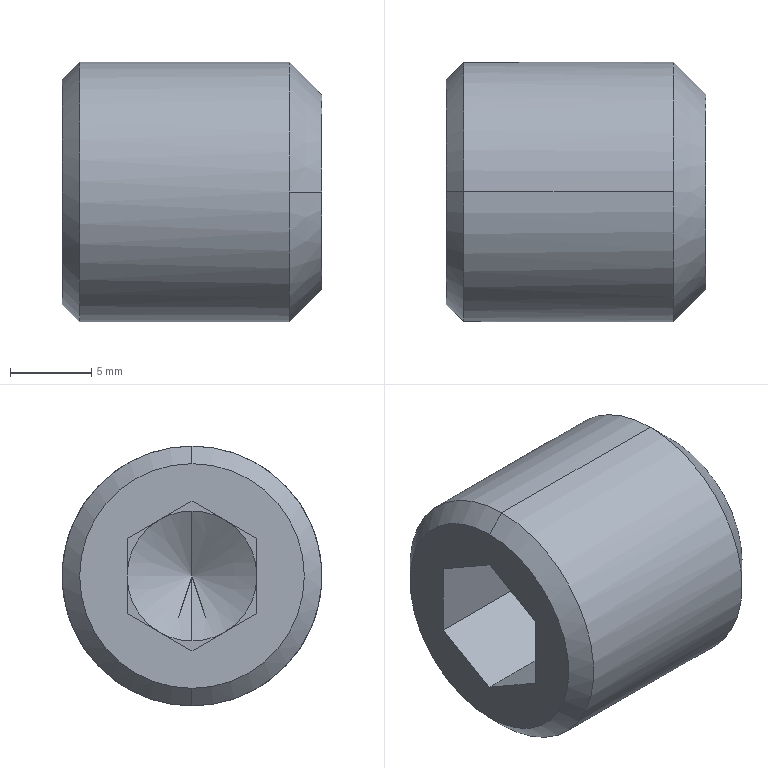Part | SolidWorks | features BaseBody 1 | 1 solid | 22 faces | box 16 x 16 x 16 mm | volume 2703 mm3 | plane 14 | cone 6 | cylinder 2 | commonest cylinder face diameters 16 x2
STEP:
#1=CARTESIAN_POINT('',(14.,8.,0.));
#2=VERTEX_POINT('',#1);
#3=CARTESIAN_POINT('',(14.,0.,-8.));
#4=VERTEX_POINT('',#3);
#5=CARTESIAN_POINT('',(14.,0.,0.));
#6=DIRECTION('',(-1.,0.,0.));
#7=DIRECTION('',(0.,0.,1.));
#8=AXIS2_PLACEMENT_3D('',#5,#6,#7);
#9=CIRCLE('',#8,8.);
#10=EDGE_CURVE('',#2,#4,#9,.T.);
#11=ORIENTED_EDGE('',*,*,#10,.T.);
#12=CARTESIAN_POINT('',(1.083,0.,-8.));
#13=VERTEX_POINT('',#12);
#14=CARTESIAN_POINT('',(-10.745,0.,-8.));
#15=DIRECTION('',(-1.,0.,0.));
#16=VECTOR('',#15,1000.);
#17=LINE('',#14,#16);
#18=EDGE_CURVE('',#4,#13,#17,.T.);
#19=ORIENTED_EDGE('',*,*,#18,.T.);
#20=CARTESIAN_POINT('',(1.083,0.,8.));
#21=VERTEX_POINT('',#20);
#22=CARTESIAN_POINT('',(1.083,0.,0.));
#23=DIRECTION('',(1.,0.,0.));
#24=DIRECTION('',(0.,0.,1.));
#25=AXIS2_PLACEMENT_3D('',#22,#23,#24);
#26=CIRCLE('',#25,8.);
#27=EDGE_CURVE('',#13,#21,#26,.T.);
#28=ORIENTED_EDGE('',*,*,#27,.T.);
#29=CARTESIAN_POINT('',(14.,0.,8.));
#30=VERTEX_POINT('',#29);
#31=CARTESIAN_POINT('',(-10.745,0.,8.));
#32=DIRECTION('',(-1.,0.,0.));
#33=VECTOR('',#32,1000.);
#34=LINE('',#31,#33);
#35=EDGE_CURVE('',#30,#21,#34,.T.);
#36=ORIENTED_EDGE('',*,*,#35,.F.);
#37=CARTESIAN_POINT('',(14.,0.,0.));
#38=DIRECTION('',(-1.,0.,0.));
#39=DIRECTION('',(0.,0.,1.));
#40=AXIS2_PLACEMENT_3D('',#37,#38,#39);
#41=CIRCLE('',#40,8.);
#42=EDGE_CURVE('',#30,#2,#41,.T.);
#43=ORIENTED_EDGE('',*,*,#42,.T.);
#44=EDGE_LOOP('',(#11,#19,#28,#36,#43));
#45=FACE_OUTER_BOUND('',#44,.T.);
#46=CARTESIAN_POINT('',(-10.745,0.,0.));
#47=DIRECTION('',(-1.,0.,0.));
#48=DIRECTION('',(0.,0.,1.));
#49=AXIS2_PLACEMENT_3D('',#46,#47,#48);
#50=CYLINDRICAL_SURFACE('',#49,8.);
#51=ADVANCED_FACE('',(#45),#50,.T.);
#52=CARTESIAN_POINT('',(16.,-6.,0.));
#53=VERTEX_POINT('',#52);
#54=CARTESIAN_POINT('',(16.,6.,0.));
#55=VERTEX_POINT('',#54);
#56=CARTESIAN_POINT('',(16.,0.,0.));
#57=DIRECTION('',(-1.,0.,0.));
#58=DIRECTION('',(0.,-1.,0.));
#59=AXIS2_PLACEMENT_3D('',#56,#57,#58);
#60=CIRCLE('',#59,6.);
#61=EDGE_CURVE('',#53,#55,#60,.T.);
#62=ORIENTED_EDGE('',*,*,#61,.T.);
#63=CARTESIAN_POINT('',(14.,8.,0.));
#64=DIRECTION('',(-0.7071,0.7071,0.));
#65=VECTOR('',#64,1000.);
#66=LINE('',#63,#65);
#67=EDGE_CURVE('',#55,#2,#66,.T.);
#68=ORIENTED_EDGE('',*,*,#67,.T.);
#69=ORIENTED_EDGE('',*,*,#42,.F.);
#70=CARTESIAN_POINT('',(14.,-8.,0.));
#71=VERTEX_POINT('',#70);
#72=CARTESIAN_POINT('',(14.,0.,0.));
#73=DIRECTION('',(-1.,0.,0.));
#74=DIRECTION('',(0.,0.,1.));
#75=AXIS2_PLACEMENT_3D('',#72,#73,#74);
#76=CIRCLE('',#75,8.);
#77=EDGE_CURVE('',#71,#30,#76,.T.);
#78=ORIENTED_EDGE('',*,*,#77,.F.);
#79=CARTESIAN_POINT('',(14.,-8.,0.));
#80=DIRECTION('',(-0.7071,-0.7071,0.));
#81=VECTOR('',#80,1000.);
#82=LINE('',#79,#81);
#83=EDGE_CURVE('',#53,#71,#82,.T.);
#84=ORIENTED_EDGE('',*,*,#83,.F.);
#85=EDGE_LOOP('',(#62,#68,#69,#78,#84));
#86=FACE_OUTER_BOUND('',#85,.T.);
#87=CARTESIAN_POINT('',(14.,0.,0.));
#88=DIRECTION('',(-1.,0.,0.));
#89=DIRECTION('',(0.,-1.,0.));
#90=AXIS2_PLACEMENT_3D('',#87,#88,#89);
#91=CONICAL_SURFACE('',#90,8.,0.7854);
#92=ADVANCED_FACE('',(#86),#91,.T.);
#93=CARTESIAN_POINT('',(0.,0.,-6.918));
#94=VERTEX_POINT('',#93);
#95=CARTESIAN_POINT('',(0.,0.,6.918));
#96=VERTEX_POINT('',#95);
#97=CARTESIAN_POINT('',(0.,0.,0.));
#98=DIRECTION('',(1.,0.,0.));
#99=DIRECTION('',(0.,0.,-1.));
#100=AXIS2_PLACEMENT_3D('',#97,#98,#99);
#101=CIRCLE('',#100,6.918);
#102=EDGE_CURVE('',#94,#96,#101,.T.);
#103=ORIENTED_EDGE('',*,*,#102,.T.);
#104=CARTESIAN_POINT('',(1.083,0.,8.));
#105=DIRECTION('',(0.7071,0.,0.7071));
#106=VECTOR('',#105,1000.);
#107=LINE('',#104,#106);
#108=EDGE_CURVE('',#96,#21,#107,.T.);
#109=ORIENTED_EDGE('',*,*,#108,.T.);
#110=ORIENTED_EDGE('',*,*,#27,.F.);
#111=CARTESIAN_POINT('',(1.083,0.,-8.));
#112=DIRECTION('',(0.7071,0.,-0.7071));
#113=VECTOR('',#112,1000.);
#114=LINE('',#111,#113);
#115=EDGE_CURVE('',#94,#13,#114,.T.);
#116=ORIENTED_EDGE('',*,*,#115,.F.);
#117=EDGE_LOOP('',(#103,#109,#110,#116));
#118=FACE_OUTER_BOUND('',#117,.T.);
#119=CARTESIAN_POINT('',(1.083,0.,0.));
#120=DIRECTION('',(1.,0.,0.));
#121=DIRECTION('',(0.,0.,-1.));
#122=AXIS2_PLACEMENT_3D('',#119,#120,#121);
#123=CONICAL_SURFACE('',#122,8.,0.7854);
#124=ADVANCED_FACE('',(#118),#123,.T.);
#125=CARTESIAN_POINT('',(8.709,0.,0.));
#126=VERTEX_POINT('',#125);
#127=CARTESIAN_POINT('',(6.4,0.,4.));
#128=VERTEX_POINT('',#127);
#129=CARTESIAN_POINT('',(6.4,0.,4.));
#130=DIRECTION('',(-0.5,0.,0.866));
#131=VECTOR('',#130,1000.);
#132=LINE('',#129,#131);
#133=EDGE_CURVE('',#126,#128,#132,.T.);
#134=ORIENTED_EDGE('',*,*,#133,.F.);
#135=CARTESIAN_POINT('',(6.4,0.,-4.));
#136=VERTEX_POINT('',#135);
#137=CARTESIAN_POINT('',(6.4,0.,-4.));
#138=DIRECTION('',(-0.5,0.,-0.866));
#139=VECTOR('',#138,1000.);
#140=LINE('',#137,#139);
#141=EDGE_CURVE('',#126,#136,#140,.T.);
#142=ORIENTED_EDGE('',*,*,#141,.T.);
#143=CARTESIAN_POINT('',(6.4,-2.,-3.464));
#144=VERTEX_POINT('',#143);
#145=CARTESIAN_POINT('',(6.4,0.,0.));
#146=DIRECTION('',(1.,0.,0.));
#147=DIRECTION('',(0.,0.,1.));
#148=AXIS2_PLACEMENT_3D('',#145,#146,#147);
#149=CIRCLE('',#148,4.);
#150=EDGE_CURVE('',#144,#136,#149,.T.);
#151=ORIENTED_EDGE('',*,*,#150,.F.);
#152=CARTESIAN_POINT('',(6.4,-4.,0.));
#153=VERTEX_POINT('',#152);
#154=CARTESIAN_POINT('',(6.4,0.,0.));
#155=DIRECTION('',(1.,0.,0.));
#156=DIRECTION('',(0.,0.,1.));
#157=AXIS2_PLACEMENT_3D('',#154,#155,#156);
#158=CIRCLE('',#157,4.);
#159=EDGE_CURVE('',#153,#144,#158,.T.);
#160=ORIENTED_EDGE('',*,*,#159,.F.);
#161=CARTESIAN_POINT('',(6.4,-2.,3.464));
#162=VERTEX_POINT('',#161);
#163=CARTESIAN_POINT('',(6.4,0.,0.));
#164=DIRECTION('',(1.,0.,0.));
#165=DIRECTION('',(0.,0.,1.));
#166=AXIS2_PLACEMENT_3D('',#163,#164,#165);
#167=CIRCLE('',#166,4.);
#168=EDGE_CURVE('',#162,#153,#167,.T.);
#169=ORIENTED_EDGE('',*,*,#168,.F.);
#170=CARTESIAN_POINT('',(6.4,0.,0.));
#171=DIRECTION('',(1.,0.,0.));
#172=DIRECTION('',(0.,0.,1.));
#173=AXIS2_PLACEMENT_3D('',#170,#171,#172);
#174=CIRCLE('',#173,4.);
#175=EDGE_CURVE('',#128,#162,#174,.T.);
#176=ORIENTED_EDGE('',*,*,#175,.F.);
#177=EDGE_LOOP('',(#134,#142,#151,#160,#169,#176));
#178=FACE_OUTER_BOUND('',#177,.T.);
#179=CARTESIAN_POINT('',(6.4,0.,0.));
#180=DIRECTION('',(-1.,0.,0.));
#181=DIRECTION('',(0.,0.,1.));
#182=AXIS2_PLACEMENT_3D('',#179,#180,#181);
#183=CONICAL_SURFACE('',#182,4.,1.047);
#184=ADVANCED_FACE('',(#178),#183,.F.);
#185=ORIENTED_EDGE('',*,*,#18,.F.);
#186=CARTESIAN_POINT('',(14.,0.,0.));
#187=DIRECTION('',(-1.,0.,0.));
#188=DIRECTION('',(0.,0.,1.));
#189=AXIS2_PLACEMENT_3D('',#186,#187,#188);
#190=CIRCLE('',#189,8.);
#191=EDGE_CURVE('',#4,#71,#190,.T.);
#192=ORIENTED_EDGE('',*,*,#191,.T.);
#193=ORIENTED_EDGE('',*,*,#77,.T.);
#194=ORIENTED_EDGE('',*,*,#35,.T.);
#195=CARTESIAN_POINT('',(1.083,0.,0.));
#196=DIRECTION('',(1.,0.,0.));
#197=DIRECTION('',(0.,0.,1.));
#198=AXIS2_PLACEMENT_3D('',#195,#196,#197);
#199=CIRCLE('',#198,8.);
#200=EDGE_CURVE('',#21,#13,#199,.T.);
#201=ORIENTED_EDGE('',*,*,#200,.T.);
#202=EDGE_LOOP('',(#185,#192,#193,#194,#201));
#203=FACE_OUTER_BOUND('',#202,.T.);
#204=CARTESIAN_POINT('',(-10.745,0.,0.));
#205=DIRECTION('',(-1.,0.,0.));
#206=DIRECTION('',(0.,0.,1.));
#207=AXIS2_PLACEMENT_3D('',#204,#205,#206);
#208=CYLINDRICAL_SURFACE('',#207,8.);
#209=ADVANCED_FACE('',(#203),#208,.T.);
#210=ORIENTED_EDGE('',*,*,#67,.F.);
#211=CARTESIAN_POINT('',(16.,0.,0.));
#212=DIRECTION('',(-1.,0.,0.));
#213=DIRECTION('',(0.,-1.,0.));
#214=AXIS2_PLACEMENT_3D('',#211,#212,#213);
#215=CIRCLE('',#214,6.);
#216=EDGE_CURVE('',#55,#53,#215,.T.);
#217=ORIENTED_EDGE('',*,*,#216,.T.);
#218=ORIENTED_EDGE('',*,*,#83,.T.);
#219=ORIENTED_EDGE('',*,*,#191,.F.);
#220=ORIENTED_EDGE('',*,*,#10,.F.);
#221=EDGE_LOOP('',(#210,#217,#218,#219,#220));
#222=FACE_OUTER_BOUND('',#221,.T.);
#223=CARTESIAN_POINT('',(14.,0.,0.));
#224=DIRECTION('',(-1.,0.,0.));
#225=DIRECTION('',(0.,-1.,0.));
#226=AXIS2_PLACEMENT_3D('',#223,#224,#225);
#227=CONICAL_SURFACE('',#226,8.,0.7854);
#228=ADVANCED_FACE('',(#222),#227,.T.);
#229=ORIENTED_EDGE('',*,*,#108,.F.);
#230=CARTESIAN_POINT('',(0.,0.,0.));
#231=DIRECTION('',(1.,0.,0.));
#232=DIRECTION('',(0.,0.,-1.));
#233=AXIS2_PLACEMENT_3D('',#230,#231,#232);
#234=CIRCLE('',#233,6.918);
#235=EDGE_CURVE('',#96,#94,#234,.T.);
#236=ORIENTED_EDGE('',*,*,#235,.T.);
#237=ORIENTED_EDGE('',*,*,#115,.T.);
#238=ORIENTED_EDGE('',*,*,#200,.F.);
#239=EDGE_LOOP('',(#229,#236,#237,#238));
#240=FACE_OUTER_BOUND('',#239,.T.);
#241=CARTESIAN_POINT('',(1.083,0.,0.));
#242=DIRECTION('',(1.,0.,0.));
#243=DIRECTION('',(0.,0.,-1.));
#244=AXIS2_PLACEMENT_3D('',#241,#242,#243);
#245=CONICAL_SURFACE('',#244,8.,0.7854);
#246=ADVANCED_FACE('',(#240),#245,.T.);
#247=ORIENTED_EDGE('',*,*,#61,.F.);
#248=ORIENTED_EDGE('',*,*,#216,.F.);
#249=EDGE_LOOP('',(#247,#248));
#250=FACE_OUTER_BOUND('',#249,.T.);
#251=CARTESIAN_POINT('',(16.,0.,0.));
#252=DIRECTION('',(-1.,0.,0.));
#253=DIRECTION('',(0.,0.,1.));
#254=AXIS2_PLACEMENT_3D('',#251,#252,#253);
#255=PLANE('',#254);
#256=ADVANCED_FACE('',(#250),#255,.F.);
#257=CARTESIAN_POINT('',(0.,-4.,-2.309));
#258=VERTEX_POINT('',#257);
#259=CARTESIAN_POINT('',(0.,-4.,2.309));
#260=VERTEX_POINT('',#259);
#261=CARTESIAN_POINT('',(0.,-4.,0.));
#262=DIRECTION('',(0.,0.,1.));
#263=VECTOR('',#262,1000.);
#264=LINE('',#261,#263);
#265=EDGE_CURVE('',#258,#260,#264,.T.);
#266=ORIENTED_EDGE('',*,*,#265,.F.);
#267=CARTESIAN_POINT('',(0.,0.,-4.619));
#268=VERTEX_POINT('',#267);
#269=CARTESIAN_POINT('',(0.,0.,-4.619));
#270=DIRECTION('',(0.,-0.866,0.5));
#271=VECTOR('',#270,1000.);
#272=LINE('',#269,#271);
#273=EDGE_CURVE('',#268,#258,#272,.T.);
#274=ORIENTED_EDGE('',*,*,#273,.F.);
#275=CARTESIAN_POINT('',(0.,4.,-2.309));
#276=VERTEX_POINT('',#275);
#277=CARTESIAN_POINT('',(0.,4.,-2.309));
#278=DIRECTION('',(0.,-0.866,-0.5));
#279=VECTOR('',#278,1000.);
#280=LINE('',#277,#279);
#281=EDGE_CURVE('',#276,#268,#280,.T.);
#282=ORIENTED_EDGE('',*,*,#281,.F.);
#283=CARTESIAN_POINT('',(0.,4.,2.309));
#284=VERTEX_POINT('',#283);
#285=CARTESIAN_POINT('',(0.,4.,0.));
#286=DIRECTION('',(0.,0.,-1.));
#287=VECTOR('',#286,1000.);
#288=LINE('',#285,#287);
#289=EDGE_CURVE('',#284,#276,#288,.T.);
#290=ORIENTED_EDGE('',*,*,#289,.F.);
#291=CARTESIAN_POINT('',(0.,0.,4.619));
#292=VERTEX_POINT('',#291);
#293=CARTESIAN_POINT('',(0.,0.,4.619));
#294=DIRECTION('',(0.,0.866,-0.5));
#295=VECTOR('',#294,1000.);
#296=LINE('',#293,#295);
#297=EDGE_CURVE('',#292,#284,#296,.T.);
#298=ORIENTED_EDGE('',*,*,#297,.F.);
#299=CARTESIAN_POINT('',(0.,-4.,2.309));
#300=DIRECTION('',(0.,0.866,0.5));
#301=VECTOR('',#300,1000.);
#302=LINE('',#299,#301);
#303=EDGE_CURVE('',#260,#292,#302,.T.);
#304=ORIENTED_EDGE('',*,*,#303,.F.);
#305=EDGE_LOOP('',(#266,#274,#282,#290,#298,#304));
#306=FACE_BOUND('',#305,.T.);
#307=ORIENTED_EDGE('',*,*,#102,.F.);
#308=ORIENTED_EDGE('',*,*,#235,.F.);
#309=EDGE_LOOP('',(#307,#308));
#310=FACE_OUTER_BOUND('',#309,.T.);
#311=CARTESIAN_POINT('',(0.,6.918,0.));
#312=DIRECTION('',(1.,0.,0.));
#313=DIRECTION('',(0.,0.,-1.));
#314=AXIS2_PLACEMENT_3D('',#311,#312,#313);
#315=PLANE('',#314);
#316=ADVANCED_FACE('',(#306,#310),#315,.F.);
#317=CARTESIAN_POINT('',(6.4,0.,4.619));
#318=VERTEX_POINT('',#317);
#319=CARTESIAN_POINT('',(6.4,-4.,2.309));
#320=DIRECTION('',(0.,0.866,0.5));
#321=VECTOR('',#320,1000.);
#322=LINE('',#319,#321);
#323=EDGE_CURVE('',#162,#318,#322,.T.);
#324=ORIENTED_EDGE('',*,*,#323,.F.);
#325=CARTESIAN_POINT('',(6.4,-4.,2.309));
#326=VERTEX_POINT('',#325);
#327=CARTESIAN_POINT('',(6.4,-4.,2.309));
#328=DIRECTION('',(0.,0.866,0.5));
#329=VECTOR('',#328,1000.);
#330=LINE('',#327,#329);
#331=EDGE_CURVE('',#326,#162,#330,.T.);
#332=ORIENTED_EDGE('',*,*,#331,.F.);
#333=CARTESIAN_POINT('',(6.4,-4.,2.309));
#334=DIRECTION('',(1.,0.,0.));
#335=VECTOR('',#334,1000.);
#336=LINE('',#333,#335);
#337=EDGE_CURVE('',#260,#326,#336,.T.);
#338=ORIENTED_EDGE('',*,*,#337,.F.);
#339=ORIENTED_EDGE('',*,*,#303,.T.);
#340=CARTESIAN_POINT('',(6.4,0.,4.619));
#341=DIRECTION('',(-1.,0.,0.));
#342=VECTOR('',#341,1000.);
#343=LINE('',#340,#342);
#344=EDGE_CURVE('',#318,#292,#343,.T.);
#345=ORIENTED_EDGE('',*,*,#344,.F.);
#346=EDGE_LOOP('',(#324,#332,#338,#339,#345));
#347=FACE_OUTER_BOUND('',#346,.T.);
#348=CARTESIAN_POINT('',(6.4,-4.,2.309));
#349=DIRECTION('',(0.,-0.5,0.866));
#350=DIRECTION('',(0.,-0.866,-0.5));
#351=AXIS2_PLACEMENT_3D('',#348,#349,#350);
#352=PLANE('',#351);
#353=ADVANCED_FACE('',(#347),#352,.F.);
#354=CARTESIAN_POINT('',(6.4,-4.,-2.309));
#355=DIRECTION('',(0.,0.,1.));
#356=VECTOR('',#355,1000.);
#357=LINE('',#354,#356);
#358=EDGE_CURVE('',#153,#326,#357,.T.);
#359=ORIENTED_EDGE('',*,*,#358,.F.);
#360=CARTESIAN_POINT('',(6.4,-4.,-2.309));
#361=VERTEX_POINT('',#360);
#362=CARTESIAN_POINT('',(6.4,-4.,-2.309));
#363=DIRECTION('',(0.,0.,1.));
#364=VECTOR('',#363,1000.);
#365=LINE('',#362,#364);
#366=EDGE_CURVE('',#361,#153,#365,.T.);
#367=ORIENTED_EDGE('',*,*,#366,.F.);
#368=CARTESIAN_POINT('',(6.4,-4.,-2.309));
#369=DIRECTION('',(1.,0.,0.));
#370=VECTOR('',#369,1000.);
#371=LINE('',#368,#370);
#372=EDGE_CURVE('',#258,#361,#371,.T.);
#373=ORIENTED_EDGE('',*,*,#372,.F.);
#374=ORIENTED_EDGE('',*,*,#265,.T.);
#375=ORIENTED_EDGE('',*,*,#337,.T.);
#376=EDGE_LOOP('',(#359,#367,#373,#374,#375));
#377=FACE_OUTER_BOUND('',#376,.T.);
#378=CARTESIAN_POINT('',(6.4,-4.,-2.309));
#379=DIRECTION('',(0.,-1.,0.));
#380=DIRECTION('',(0.,0.,-1.));
#381=AXIS2_PLACEMENT_3D('',#378,#379,#380);
#382=PLANE('',#381);
#383=ADVANCED_FACE('',(#377),#382,.F.);
#384=CARTESIAN_POINT('',(6.4,0.,-4.619));
#385=DIRECTION('',(0.,-0.866,0.5));
#386=VECTOR('',#385,1000.);
#387=LINE('',#384,#386);
#388=EDGE_CURVE('',#144,#361,#387,.T.);
#389=ORIENTED_EDGE('',*,*,#388,.F.);
#390=CARTESIAN_POINT('',(6.4,0.,-4.619));
#391=VERTEX_POINT('',#390);
#392=CARTESIAN_POINT('',(6.4,0.,-4.619));
#393=DIRECTION('',(0.,-0.866,0.5));
#394=VECTOR('',#393,1000.);
#395=LINE('',#392,#394);
#396=EDGE_CURVE('',#391,#144,#395,.T.);
#397=ORIENTED_EDGE('',*,*,#396,.F.);
#398=CARTESIAN_POINT('',(6.4,0.,-4.619));
#399=DIRECTION('',(1.,0.,0.));
#400=VECTOR('',#399,1000.);
#401=LINE('',#398,#400);
#402=EDGE_CURVE('',#268,#391,#401,.T.);
#403=ORIENTED_EDGE('',*,*,#402,.F.);
#404=ORIENTED_EDGE('',*,*,#273,.T.);
#405=ORIENTED_EDGE('',*,*,#372,.T.);
#406=EDGE_LOOP('',(#389,#397,#403,#404,#405));
#407=FACE_OUTER_BOUND('',#406,.T.);
#408=CARTESIAN_POINT('',(6.4,0.,-4.619));
#409=DIRECTION('',(0.,-0.5,-0.866));
#410=DIRECTION('',(0.,0.866,-0.5));
#411=AXIS2_PLACEMENT_3D('',#408,#409,#410);
#412=PLANE('',#411);
#413=ADVANCED_FACE('',(#407),#412,.F.);
#414=CARTESIAN_POINT('',(6.4,2.,-3.464));
#415=VERTEX_POINT('',#414);
#416=CARTESIAN_POINT('',(6.4,4.,-2.309));
#417=DIRECTION('',(0.,-0.866,-0.5));
#418=VECTOR('',#417,1000.);
#419=LINE('',#416,#418);
#420=EDGE_CURVE('',#415,#391,#419,.T.);
#421=ORIENTED_EDGE('',*,*,#420,.F.);
#422=CARTESIAN_POINT('',(6.4,4.,-2.309));
#423=VERTEX_POINT('',#422);
#424=CARTESIAN_POINT('',(6.4,4.,-2.309));
#425=DIRECTION('',(0.,-0.866,-0.5));
#426=VECTOR('',#425,1000.);
#427=LINE('',#424,#426);
#428=EDGE_CURVE('',#423,#415,#427,.T.);
#429=ORIENTED_EDGE('',*,*,#428,.F.);
#430=CARTESIAN_POINT('',(6.4,4.,-2.309));
#431=DIRECTION('',(1.,0.,0.));
#432=VECTOR('',#431,1000.);
#433=LINE('',#430,#432);
#434=EDGE_CURVE('',#276,#423,#433,.T.);
#435=ORIENTED_EDGE('',*,*,#434,.F.);
#436=ORIENTED_EDGE('',*,*,#281,.T.);
#437=ORIENTED_EDGE('',*,*,#402,.T.);
#438=EDGE_LOOP('',(#421,#429,#435,#436,#437));
#439=FACE_OUTER_BOUND('',#438,.T.);
#440=CARTESIAN_POINT('',(6.4,4.,-2.309));
#441=DIRECTION('',(0.,0.5,-0.866));
#442=DIRECTION('',(0.,0.866,0.5));
#443=AXIS2_PLACEMENT_3D('',#440,#441,#442);
#444=PLANE('',#443);
#445=ADVANCED_FACE('',(#439),#444,.F.);
#446=CARTESIAN_POINT('',(6.4,4.,0.));
#447=VERTEX_POINT('',#446);
#448=CARTESIAN_POINT('',(6.4,4.,2.309));
#449=DIRECTION('',(0.,0.,-1.));
#450=VECTOR('',#449,1000.);
#451=LINE('',#448,#450);
#452=EDGE_CURVE('',#447,#423,#451,.T.);
#453=ORIENTED_EDGE('',*,*,#452,.F.);
#454=CARTESIAN_POINT('',(6.4,4.,2.309));
#455=VERTEX_POINT('',#454);
#456=CARTESIAN_POINT('',(6.4,4.,2.309));
#457=DIRECTION('',(0.,0.,-1.));
#458=VECTOR('',#457,1000.);
#459=LINE('',#456,#458);
#460=EDGE_CURVE('',#455,#447,#459,.T.);
#461=ORIENTED_EDGE('',*,*,#460,.F.);
#462=CARTESIAN_POINT('',(6.4,4.,2.309));
#463=DIRECTION('',(1.,0.,0.));
#464=VECTOR('',#463,1000.);
#465=LINE('',#462,#464);
#466=EDGE_CURVE('',#284,#455,#465,.T.);
#467=ORIENTED_EDGE('',*,*,#466,.F.);
#468=ORIENTED_EDGE('',*,*,#289,.T.);
#469=ORIENTED_EDGE('',*,*,#434,.T.);
#470=EDGE_LOOP('',(#453,#461,#467,#468,#469));
#471=FACE_OUTER_BOUND('',#470,.T.);
#472=CARTESIAN_POINT('',(6.4,4.,2.309));
#473=DIRECTION('',(0.,1.,0.));
#474=DIRECTION('',(0.,0.,1.));
#475=AXIS2_PLACEMENT_3D('',#472,#473,#474);
#476=PLANE('',#475);
#477=ADVANCED_FACE('',(#471),#476,.F.);
#478=CARTESIAN_POINT('',(6.4,2.,3.464));
#479=VERTEX_POINT('',#478);
#480=CARTESIAN_POINT('',(6.4,0.,4.619));
#481=DIRECTION('',(0.,0.866,-0.5));
#482=VECTOR('',#481,1000.);
#483=LINE('',#480,#482);
#484=EDGE_CURVE('',#479,#455,#483,.T.);
#485=ORIENTED_EDGE('',*,*,#484,.F.);
#486=CARTESIAN_POINT('',(6.4,0.,4.619));
#487=DIRECTION('',(0.,0.866,-0.5));
#488=VECTOR('',#487,1000.);
#489=LINE('',#486,#488);
#490=EDGE_CURVE('',#318,#479,#489,.T.);
#491=ORIENTED_EDGE('',*,*,#490,.F.);
#492=ORIENTED_EDGE('',*,*,#344,.T.);
#493=ORIENTED_EDGE('',*,*,#297,.T.);
#494=ORIENTED_EDGE('',*,*,#466,.T.);
#495=EDGE_LOOP('',(#485,#491,#492,#493,#494));
#496=FACE_OUTER_BOUND('',#495,.T.);
#497=CARTESIAN_POINT('',(6.4,0.,4.619));
#498=DIRECTION('',(0.,0.5,0.866));
#499=DIRECTION('',(0.,-0.866,0.5));
#500=AXIS2_PLACEMENT_3D('',#497,#498,#499);
#501=PLANE('',#500);
#502=ADVANCED_FACE('',(#496),#501,.F.);
#503=ORIENTED_EDGE('',*,*,#490,.T.);
#504=CARTESIAN_POINT('',(6.4,0.,0.));
#505=DIRECTION('',(1.,0.,0.));
#506=DIRECTION('',(0.,0.,1.));
#507=AXIS2_PLACEMENT_3D('',#504,#505,#506);
#508=CIRCLE('',#507,4.);
#509=EDGE_CURVE('',#479,#128,#508,.T.);
#510=ORIENTED_EDGE('',*,*,#509,.T.);
#511=ORIENTED_EDGE('',*,*,#175,.T.);
#512=ORIENTED_EDGE('',*,*,#323,.T.);
#513=EDGE_LOOP('',(#503,#510,#511,#512));
#514=FACE_OUTER_BOUND('',#513,.T.);
#515=CARTESIAN_POINT('',(6.4,0.,4.619));
#516=DIRECTION('',(-1.,0.,0.));
#517=DIRECTION('',(0.,0.,1.));
#518=AXIS2_PLACEMENT_3D('',#515,#516,#517);
#519=PLANE('',#518);
#520=ADVANCED_FACE('',(#514),#519,.T.);
#521=ORIENTED_EDGE('',*,*,#331,.T.);
#522=ORIENTED_EDGE('',*,*,#168,.T.);
#523=ORIENTED_EDGE('',*,*,#358,.T.);
#524=EDGE_LOOP('',(#521,#522,#523));
#525=FACE_OUTER_BOUND('',#524,.T.);
#526=CARTESIAN_POINT('',(6.4,0.,4.619));
#527=DIRECTION('',(-1.,0.,0.));
#528=DIRECTION('',(0.,0.,1.));
#529=AXIS2_PLACEMENT_3D('',#526,#527,#528);
#530=PLANE('',#529);
#531=ADVANCED_FACE('',(#525),#530,.T.);
#532=ORIENTED_EDGE('',*,*,#366,.T.);
#533=ORIENTED_EDGE('',*,*,#159,.T.);
#534=ORIENTED_EDGE('',*,*,#388,.T.);
#535=EDGE_LOOP('',(#532,#533,#534));
#536=FACE_OUTER_BOUND('',#535,.T.);
#537=CARTESIAN_POINT('',(6.4,0.,4.619));
#538=DIRECTION('',(-1.,0.,0.));
#539=DIRECTION('',(0.,0.,1.));
#540=AXIS2_PLACEMENT_3D('',#537,#538,#539);
#541=PLANE('',#540);
#542=ADVANCED_FACE('',(#536),#541,.T.);
#543=ORIENTED_EDGE('',*,*,#396,.T.);
#544=ORIENTED_EDGE('',*,*,#150,.T.);
#545=CARTESIAN_POINT('',(6.4,0.,0.));
#546=DIRECTION('',(1.,0.,0.));
#547=DIRECTION('',(0.,0.,1.));
#548=AXIS2_PLACEMENT_3D('',#545,#546,#547);
#549=CIRCLE('',#548,4.);
#550=EDGE_CURVE('',#136,#415,#549,.T.);
#551=ORIENTED_EDGE('',*,*,#550,.T.);
#552=ORIENTED_EDGE('',*,*,#420,.T.);
#553=EDGE_LOOP('',(#543,#544,#551,#552));
#554=FACE_OUTER_BOUND('',#553,.T.);
#555=CARTESIAN_POINT('',(6.4,0.,4.619));
#556=DIRECTION('',(-1.,0.,0.));
#557=DIRECTION('',(0.,0.,1.));
#558=AXIS2_PLACEMENT_3D('',#555,#556,#557);
#559=PLANE('',#558);
#560=ADVANCED_FACE('',(#554),#559,.T.);
#561=ORIENTED_EDGE('',*,*,#428,.T.);
#562=CARTESIAN_POINT('',(6.4,0.,0.));
#563=DIRECTION('',(1.,0.,0.));
#564=DIRECTION('',(0.,0.,1.));
#565=AXIS2_PLACEMENT_3D('',#562,#563,#564);
#566=CIRCLE('',#565,4.);
#567=EDGE_CURVE('',#415,#447,#566,.T.);
#568=ORIENTED_EDGE('',*,*,#567,.T.);
#569=ORIENTED_EDGE('',*,*,#452,.T.);
#570=EDGE_LOOP('',(#561,#568,#569));
#571=FACE_OUTER_BOUND('',#570,.T.);
#572=CARTESIAN_POINT('',(6.4,0.,4.619));
#573=DIRECTION('',(-1.,0.,0.));
#574=DIRECTION('',(0.,0.,1.));
#575=AXIS2_PLACEMENT_3D('',#572,#573,#574);
#576=PLANE('',#575);
#577=ADVANCED_FACE('',(#571),#576,.T.);
#578=ORIENTED_EDGE('',*,*,#460,.T.);
#579=CARTESIAN_POINT('',(6.4,0.,0.));
#580=DIRECTION('',(1.,0.,0.));
#581=DIRECTION('',(0.,0.,1.));
#582=AXIS2_PLACEMENT_3D('',#579,#580,#581);
#583=CIRCLE('',#582,4.);
#584=EDGE_CURVE('',#447,#479,#583,.T.);
#585=ORIENTED_EDGE('',*,*,#584,.T.);
#586=ORIENTED_EDGE('',*,*,#484,.T.);
#587=EDGE_LOOP('',(#578,#585,#586));
#588=FACE_OUTER_BOUND('',#587,.T.);
#589=CARTESIAN_POINT('',(6.4,0.,4.619));
#590=DIRECTION('',(-1.,0.,0.));
#591=DIRECTION('',(0.,0.,1.));
#592=AXIS2_PLACEMENT_3D('',#589,#590,#591);
#593=PLANE('',#592);
#594=ADVANCED_FACE('',(#588),#593,.T.);
#595=ORIENTED_EDGE('',*,*,#141,.F.);
#596=ORIENTED_EDGE('',*,*,#133,.T.);
#597=ORIENTED_EDGE('',*,*,#509,.F.);
#598=ORIENTED_EDGE('',*,*,#584,.F.);
#599=ORIENTED_EDGE('',*,*,#567,.F.);
#600=ORIENTED_EDGE('',*,*,#550,.F.);
#601=EDGE_LOOP('',(#595,#596,#597,#598,#599,#600));
#602=FACE_OUTER_BOUND('',#601,.T.);
#603=CARTESIAN_POINT('',(6.4,0.,0.));
#604=DIRECTION('',(-1.,0.,0.));
#605=DIRECTION('',(0.,0.,1.));
#606=AXIS2_PLACEMENT_3D('',#603,#604,#605);
#607=CONICAL_SURFACE('',#606,4.,1.047);
#608=ADVANCED_FACE('',(#602),#607,.F.);
#609=CLOSED_SHELL('',(#51,#92,#124,#184,#209,#228,#246,#256,#316,#353,#383,#413,#445,#477,#502,#520,#531,#542,#560,#577,#594,#608));
#610=MANIFOLD_SOLID_BREP('',#609);
#611=CARTESIAN_POINT('',(0.,0.,0.));
#612=DIRECTION('',(0.,0.,1.));
#613=DIRECTION('',(1.,0.,0.));
#614=AXIS2_PLACEMENT_3D('',#611,#612,#613);
#615=(LENGTH_UNIT()NAMED_UNIT(*)SI_UNIT(.MILLI.,.METRE.));
#616=UNCERTAINTY_MEASURE_WITH_UNIT(LENGTH_MEASURE(0.00001),#615,'','');
#617=(NAMED_UNIT(*)PLANE_ANGLE_UNIT()SI_UNIT($,.RADIAN.));
#618=(NAMED_UNIT(*)SI_UNIT($,.STERADIAN.)SOLID_ANGLE_UNIT());
#619=(GEOMETRIC_REPRESENTATION_CONTEXT(3)GLOBAL_UNCERTAINTY_ASSIGNED_CONTEXT((#616))GLOBAL_UNIT_ASSIGNED_CONTEXT((#615,#617,#618))REPRESENTATION_CONTEXT('',''));
#620=ADVANCED_BREP_SHAPE_REPRESENTATION('',(#610,#614),#619);